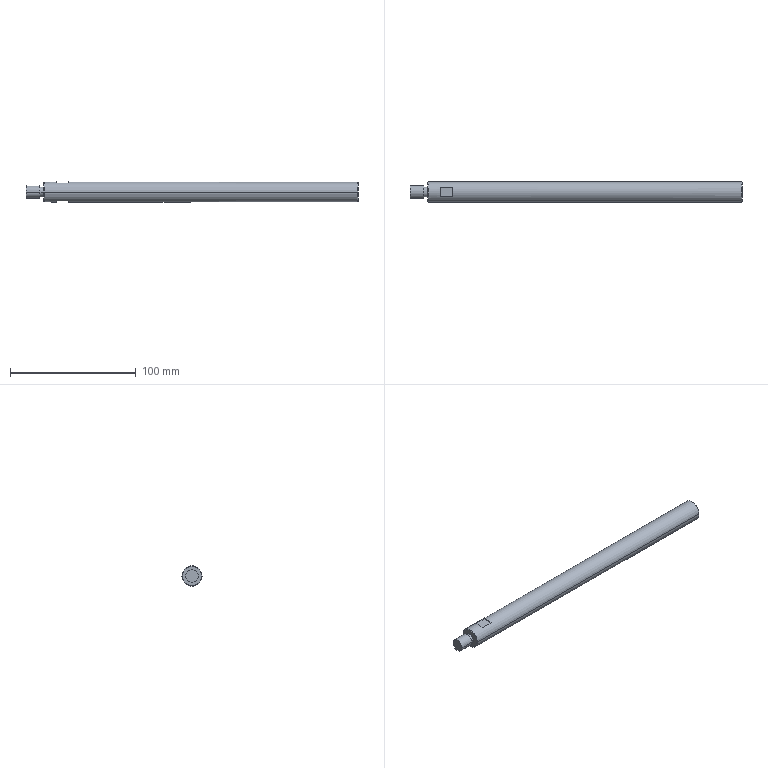Part | STEP file | PSSAGS16-250-F14-M10-SC10 | 1 solid | 20 faces | box 264 x 16 x 16 mm | volume 51157 mm3 | plane 10 | cylinder 6 | cone 4 | commonest cylinder face diameters 7.7 x2 10 x2 16 x2
STEP:
#1=CARTESIAN_POINT('',(0.,0.,0.));
#2=DIRECTION('',(0.,0.,1.));
#3=DIRECTION('',(1.,0.,0.));
#4=AXIS2_PLACEMENT_3D('',#1,#2,#3);
#5=CARTESIAN_POINT('',(264.,7.6,0.));
#6=VERTEX_POINT('',#5);
#7=CARTESIAN_POINT('',(264.,-7.6,0.));
#8=VERTEX_POINT('',#7);
#9=CARTESIAN_POINT('',(264.,0.,0.));
#10=DIRECTION('',(1.,0.,0.));
#11=DIRECTION('',(0.,-1.,0.));
#12=AXIS2_PLACEMENT_3D('',#9,#10,#11);
#13=CIRCLE('',#12,7.6);
#14=CARTESIAN_POINT('',(263.6,0.,0.));
#15=DIRECTION('',(-1.,0.,0.));
#16=DIRECTION('',(0.,-1.,0.));
#17=AXIS2_PLACEMENT_3D('',#14,#15,#16);
#18=CONICAL_SURFACE('',#17,8.,0.7854);
#19=CARTESIAN_POINT('',(6.283,-0.4));
#20=DIRECTION('',(-1.,0.));
#21=VECTOR('',#20,1.);
#22=LINE('',#19,#21);
#23=(GEOMETRIC_REPRESENTATION_CONTEXT(2)PARAMETRIC_REPRESENTATION_CONTEXT()REPRESENTATION_CONTEXT('',''));
#24=DEFINITIONAL_REPRESENTATION('',(#22),#23);
#25=PCURVE('',#18,#24);
#26=CARTESIAN_POINT('',(264.,8.,0.));
#27=DIRECTION('',(-1.,0.,0.));
#28=DIRECTION('',(0.,-1.,0.));
#29=AXIS2_PLACEMENT_3D('',#26,#27,#28);
#30=PLANE('',#29);
#31=CARTESIAN_POINT('',(15.6,0.));
#32=CARTESIAN_POINT('',(15.6,-13.164));
#33=CARTESIAN_POINT('',(4.2,-6.582));
#34=CARTESIAN_POINT('',(-7.2,0.));
#35=CARTESIAN_POINT('',(4.2,6.582));
#36=CARTESIAN_POINT('',(15.6,13.164));
#37=CARTESIAN_POINT('',(15.6,0.));
#38=(BOUNDED_CURVE()B_SPLINE_CURVE(2,(#31,#32,#33,#34,#35,#36,#37),.UNSPECIFIED.,.T.,.F.)B_SPLINE_CURVE_WITH_KNOTS((1,2,2,2,2,1),(-2.094,0.,2.094,4.189,6.283,8.378),.UNSPECIFIED.)CURVE()GEOMETRIC_REPRESENTATION_ITEM()RATIONAL_B_SPLINE_CURVE((1.,0.5,1.,0.5,1.,0.5,1.))REPRESENTATION_ITEM(''));
#39=(GEOMETRIC_REPRESENTATION_CONTEXT(2)PARAMETRIC_REPRESENTATION_CONTEXT()REPRESENTATION_CONTEXT('',''));
#40=DEFINITIONAL_REPRESENTATION('',(#38),#39);
#41=PCURVE('',#30,#40);
#42=SURFACE_CURVE('',#13,(#25,#41),.PCURVE_S1.);
#43=EDGE_CURVE('',#6,#8,#42,.T.);
#44=ORIENTED_EDGE('',*,*,#43,.F.);
#45=CARTESIAN_POINT('',(263.6,8.,0.));
#46=VERTEX_POINT('',#45);
#47=CARTESIAN_POINT('',(263.6,8.,0.));
#48=DIRECTION('',(-0.7071,0.7071,0.));
#49=VECTOR('',#48,1.);
#50=LINE('',#47,#49);
#51=CARTESIAN_POINT('',(3.142,0.));
#52=DIRECTION('',(0.,1.));
#53=VECTOR('',#52,1.);
#54=LINE('',#51,#53);
#55=(GEOMETRIC_REPRESENTATION_CONTEXT(2)PARAMETRIC_REPRESENTATION_CONTEXT()REPRESENTATION_CONTEXT('',''));
#56=DEFINITIONAL_REPRESENTATION('',(#54),#55);
#57=PCURVE('',#18,#56);
#58=CARTESIAN_POINT('',(263.6,0.,0.));
#59=DIRECTION('',(-1.,0.,0.));
#60=DIRECTION('',(0.,-1.,0.));
#61=AXIS2_PLACEMENT_3D('',#58,#59,#60);
#62=CONICAL_SURFACE('',#61,8.,0.7854);
#63=CARTESIAN_POINT('',(3.142,0.));
#64=DIRECTION('',(0.,1.));
#65=VECTOR('',#64,1.);
#66=LINE('',#63,#65);
#67=(GEOMETRIC_REPRESENTATION_CONTEXT(2)PARAMETRIC_REPRESENTATION_CONTEXT()REPRESENTATION_CONTEXT('',''));
#68=DEFINITIONAL_REPRESENTATION('',(#66),#67);
#69=PCURVE('',#62,#68);
#70=SURFACE_CURVE('',#50,(#57,#69),.PCURVE_S1.);
#71=EDGE_CURVE('',#6,#46,#70,.T.);
#72=ORIENTED_EDGE('',*,*,#71,.T.);
#73=CARTESIAN_POINT('',(263.6,-8.,0.));
#74=VERTEX_POINT('',#73);
#75=CARTESIAN_POINT('',(263.6,0.,0.));
#76=DIRECTION('',(-1.,0.,0.));
#77=DIRECTION('',(0.,-1.,0.));
#78=AXIS2_PLACEMENT_3D('',#75,#76,#77);
#79=CIRCLE('',#78,8.);
#80=CARTESIAN_POINT('',(0.,0.));
#81=DIRECTION('',(1.,0.));
#82=VECTOR('',#81,1.);
#83=LINE('',#80,#82);
#84=(GEOMETRIC_REPRESENTATION_CONTEXT(2)PARAMETRIC_REPRESENTATION_CONTEXT()REPRESENTATION_CONTEXT('',''));
#85=DEFINITIONAL_REPRESENTATION('',(#83),#84);
#86=PCURVE('',#18,#85);
#87=CARTESIAN_POINT('',(0.,0.,0.));
#88=DIRECTION('',(-1.,0.,0.));
#89=DIRECTION('',(0.,-1.,0.));
#90=AXIS2_PLACEMENT_3D('',#87,#88,#89);
#91=CYLINDRICAL_SURFACE('',#90,8.);
#92=CARTESIAN_POINT('',(0.,-263.6));
#93=DIRECTION('',(1.,0.));
#94=VECTOR('',#93,1.);
#95=LINE('',#92,#94);
#96=(GEOMETRIC_REPRESENTATION_CONTEXT(2)PARAMETRIC_REPRESENTATION_CONTEXT()REPRESENTATION_CONTEXT('',''));
#97=DEFINITIONAL_REPRESENTATION('',(#95),#96);
#98=PCURVE('',#91,#97);
#99=SURFACE_CURVE('',#79,(#86,#98),.PCURVE_S1.);
#100=EDGE_CURVE('',#74,#46,#99,.T.);
#101=ORIENTED_EDGE('',*,*,#100,.F.);
#102=CARTESIAN_POINT('',(263.6,-8.,0.));
#103=DIRECTION('',(-0.7071,-0.7071,0.));
#104=VECTOR('',#103,1.);
#105=LINE('',#102,#104);
#106=CARTESIAN_POINT('',(0.,0.));
#107=DIRECTION('',(0.,1.));
#108=VECTOR('',#107,1.);
#109=LINE('',#106,#108);
#110=(GEOMETRIC_REPRESENTATION_CONTEXT(2)PARAMETRIC_REPRESENTATION_CONTEXT()REPRESENTATION_CONTEXT('',''));
#111=DEFINITIONAL_REPRESENTATION('',(#109),#110);
#112=PCURVE('',#18,#111);
#113=CARTESIAN_POINT('',(6.283,0.));
#114=DIRECTION('',(0.,1.));
#115=VECTOR('',#114,1.);
#116=LINE('',#113,#115);
#117=(GEOMETRIC_REPRESENTATION_CONTEXT(2)PARAMETRIC_REPRESENTATION_CONTEXT()REPRESENTATION_CONTEXT('',''));
#118=DEFINITIONAL_REPRESENTATION('',(#116),#117);
#119=PCURVE('',#62,#118);
#120=SURFACE_CURVE('',#105,(#112,#119),.PCURVE_S1.);
#121=EDGE_CURVE('',#8,#74,#120,.T.);
#122=ORIENTED_EDGE('',*,*,#121,.F.);
#123=EDGE_LOOP('',(#44,#72,#101,#122));
#124=FACE_BOUND('',#123,.T.);
#125=ADVANCED_FACE('',(#124),#18,.T.);
#126=CARTESIAN_POINT('',(14.,-7.6,0.));
#127=VERTEX_POINT('',#126);
#128=CARTESIAN_POINT('',(14.,7.6,0.));
#129=VERTEX_POINT('',#128);
#130=CARTESIAN_POINT('',(14.,0.,0.));
#131=DIRECTION('',(-1.,0.,0.));
#132=DIRECTION('',(0.,1.,0.));
#133=AXIS2_PLACEMENT_3D('',#130,#131,#132);
#134=CIRCLE('',#133,7.6);
#135=CARTESIAN_POINT('',(14.,0.,0.));
#136=DIRECTION('',(1.,0.,0.));
#137=DIRECTION('',(0.,1.,0.));
#138=AXIS2_PLACEMENT_3D('',#135,#136,#137);
#139=CONICAL_SURFACE('',#138,7.6,0.7854);
#140=CARTESIAN_POINT('',(6.283,0.));
#141=DIRECTION('',(-1.,0.));
#142=VECTOR('',#141,1.);
#143=LINE('',#140,#142);
#144=(GEOMETRIC_REPRESENTATION_CONTEXT(2)PARAMETRIC_REPRESENTATION_CONTEXT()REPRESENTATION_CONTEXT('',''));
#145=DEFINITIONAL_REPRESENTATION('',(#143),#144);
#146=PCURVE('',#139,#145);
#147=CARTESIAN_POINT('',(14.,3.85,0.));
#148=DIRECTION('',(1.,0.,0.));
#149=DIRECTION('',(0.,1.,0.));
#150=AXIS2_PLACEMENT_3D('',#147,#148,#149);
#151=PLANE('',#150);
#152=CARTESIAN_POINT('',(3.75,0.));
#153=CARTESIAN_POINT('',(3.75,-13.164));
#154=CARTESIAN_POINT('',(-7.65,-6.582));
#155=CARTESIAN_POINT('',(-19.05,0.));
#156=CARTESIAN_POINT('',(-7.65,6.582));
#157=CARTESIAN_POINT('',(3.75,13.164));
#158=CARTESIAN_POINT('',(3.75,0.));
#159=(BOUNDED_CURVE()B_SPLINE_CURVE(2,(#152,#153,#154,#155,#156,#157,#158),.UNSPECIFIED.,.T.,.F.)B_SPLINE_CURVE_WITH_KNOTS((1,2,2,2,2,1),(-2.094,0.,2.094,4.189,6.283,8.378),.UNSPECIFIED.)CURVE()GEOMETRIC_REPRESENTATION_ITEM()RATIONAL_B_SPLINE_CURVE((1.,0.5,1.,0.5,1.,0.5,1.))REPRESENTATION_ITEM(''));
#160=(GEOMETRIC_REPRESENTATION_CONTEXT(2)PARAMETRIC_REPRESENTATION_CONTEXT()REPRESENTATION_CONTEXT('',''));
#161=DEFINITIONAL_REPRESENTATION('',(#159),#160);
#162=PCURVE('',#151,#161);
#163=SURFACE_CURVE('',#134,(#146,#162),.PCURVE_S1.);
#164=EDGE_CURVE('',#127,#129,#163,.T.);
#165=ORIENTED_EDGE('',*,*,#164,.F.);
#166=CARTESIAN_POINT('',(14.4,-8.,0.));
#167=VERTEX_POINT('',#166);
#168=CARTESIAN_POINT('',(14.,-7.6,0.));
#169=DIRECTION('',(0.7071,-0.7071,0.));
#170=VECTOR('',#169,1.);
#171=LINE('',#168,#170);
#172=CARTESIAN_POINT('',(3.142,0.));
#173=DIRECTION('',(0.,1.));
#174=VECTOR('',#173,1.);
#175=LINE('',#172,#174);
#176=(GEOMETRIC_REPRESENTATION_CONTEXT(2)PARAMETRIC_REPRESENTATION_CONTEXT()REPRESENTATION_CONTEXT('',''));
#177=DEFINITIONAL_REPRESENTATION('',(#175),#176);
#178=PCURVE('',#139,#177);
#179=CARTESIAN_POINT('',(14.,0.,0.));
#180=DIRECTION('',(1.,0.,0.));
#181=DIRECTION('',(0.,1.,0.));
#182=AXIS2_PLACEMENT_3D('',#179,#180,#181);
#183=CONICAL_SURFACE('',#182,7.6,0.7854);
#184=CARTESIAN_POINT('',(3.142,0.));
#185=DIRECTION('',(0.,1.));
#186=VECTOR('',#185,1.);
#187=LINE('',#184,#186);
#188=(GEOMETRIC_REPRESENTATION_CONTEXT(2)PARAMETRIC_REPRESENTATION_CONTEXT()REPRESENTATION_CONTEXT('',''));
#189=DEFINITIONAL_REPRESENTATION('',(#187),#188);
#190=PCURVE('',#183,#189);
#191=SURFACE_CURVE('',#171,(#178,#190),.PCURVE_S1.);
#192=EDGE_CURVE('',#127,#167,#191,.T.);
#193=ORIENTED_EDGE('',*,*,#192,.T.);
#194=CARTESIAN_POINT('',(14.4,8.,0.));
#195=VERTEX_POINT('',#194);
#196=CARTESIAN_POINT('',(14.4,0.,0.));
#197=DIRECTION('',(1.,0.,0.));
#198=DIRECTION('',(0.,1.,0.));
#199=AXIS2_PLACEMENT_3D('',#196,#197,#198);
#200=CIRCLE('',#199,8.);
#201=CARTESIAN_POINT('',(0.,0.4));
#202=DIRECTION('',(1.,0.));
#203=VECTOR('',#202,1.);
#204=LINE('',#201,#203);
#205=(GEOMETRIC_REPRESENTATION_CONTEXT(2)PARAMETRIC_REPRESENTATION_CONTEXT()REPRESENTATION_CONTEXT('',''));
#206=DEFINITIONAL_REPRESENTATION('',(#204),#205);
#207=PCURVE('',#139,#206);
#208=CARTESIAN_POINT('',(3.142,-14.4));
#209=DIRECTION('',(-1.,0.));
#210=VECTOR('',#209,1.);
#211=LINE('',#208,#210);
#212=(GEOMETRIC_REPRESENTATION_CONTEXT(2)PARAMETRIC_REPRESENTATION_CONTEXT()REPRESENTATION_CONTEXT('',''));
#213=DEFINITIONAL_REPRESENTATION('',(#211),#212);
#214=PCURVE('',#91,#213);
#215=SURFACE_CURVE('',#200,(#207,#214),.PCURVE_S1.);
#216=EDGE_CURVE('',#195,#167,#215,.T.);
#217=ORIENTED_EDGE('',*,*,#216,.F.);
#218=CARTESIAN_POINT('',(14.,7.6,0.));
#219=DIRECTION('',(0.7071,0.7071,0.));
#220=VECTOR('',#219,1.);
#221=LINE('',#218,#220);
#222=CARTESIAN_POINT('',(0.,0.));
#223=DIRECTION('',(0.,1.));
#224=VECTOR('',#223,1.);
#225=LINE('',#222,#224);
#226=(GEOMETRIC_REPRESENTATION_CONTEXT(2)PARAMETRIC_REPRESENTATION_CONTEXT()REPRESENTATION_CONTEXT('',''));
#227=DEFINITIONAL_REPRESENTATION('',(#225),#226);
#228=PCURVE('',#139,#227);
#229=CARTESIAN_POINT('',(6.283,0.));
#230=DIRECTION('',(0.,1.));
#231=VECTOR('',#230,1.);
#232=LINE('',#229,#231);
#233=(GEOMETRIC_REPRESENTATION_CONTEXT(2)PARAMETRIC_REPRESENTATION_CONTEXT()REPRESENTATION_CONTEXT('',''));
#234=DEFINITIONAL_REPRESENTATION('',(#232),#233);
#235=PCURVE('',#183,#234);
#236=SURFACE_CURVE('',#221,(#228,#235),.PCURVE_S1.);
#237=EDGE_CURVE('',#129,#195,#236,.T.);
#238=ORIENTED_EDGE('',*,*,#237,.F.);
#239=EDGE_LOOP('',(#165,#193,#217,#238));
#240=FACE_BOUND('',#239,.T.);
#241=ADVANCED_FACE('',(#240),#139,.T.);
#242=CARTESIAN_POINT('',(24.,3.873,7.));
#243=VERTEX_POINT('',#242);
#244=CARTESIAN_POINT('',(34.,3.873,7.));
#245=VERTEX_POINT('',#244);
#246=CARTESIAN_POINT('',(0.,3.873,7.));
#247=DIRECTION('',(1.,0.,0.));
#248=VECTOR('',#247,1.);
#249=LINE('',#246,#248);
#250=CARTESIAN_POINT('',(2.076,0.));
#251=DIRECTION('',(0.,-1.));
#252=VECTOR('',#251,1.);
#253=LINE('',#250,#252);
#254=(GEOMETRIC_REPRESENTATION_CONTEXT(2)PARAMETRIC_REPRESENTATION_CONTEXT()REPRESENTATION_CONTEXT('',''));
#255=DEFINITIONAL_REPRESENTATION('',(#253),#254);
#256=PCURVE('',#91,#255);
#257=CARTESIAN_POINT('',(24.,-8.,7.));
#258=DIRECTION('',(0.,0.,-1.));
#259=DIRECTION('',(-1.,0.,0.));
#260=AXIS2_PLACEMENT_3D('',#257,#258,#259);
#261=PLANE('',#260);
#262=CARTESIAN_POINT('',(24.,11.873));
#263=DIRECTION('',(-1.,0.));
#264=VECTOR('',#263,1.);
#265=LINE('',#262,#264);
#266=(GEOMETRIC_REPRESENTATION_CONTEXT(2)PARAMETRIC_REPRESENTATION_CONTEXT()REPRESENTATION_CONTEXT('',''));
#267=DEFINITIONAL_REPRESENTATION('',(#265),#266);
#268=PCURVE('',#261,#267);
#269=SURFACE_CURVE('',#249,(#256,#268),.PCURVE_S1.);
#270=EDGE_CURVE('',#243,#245,#269,.T.);
#271=ORIENTED_EDGE('',*,*,#270,.T.);
#272=CARTESIAN_POINT('',(34.,-3.873,7.));
#273=VERTEX_POINT('',#272);
#274=CARTESIAN_POINT('',(34.,0.,0.));
#275=DIRECTION('',(1.,0.,0.));
#276=DIRECTION('',(0.,0.,-1.));
#277=AXIS2_PLACEMENT_3D('',#274,#275,#276);
#278=CIRCLE('',#277,8.);
#279=CARTESIAN_POINT('',(4.712,-34.));
#280=DIRECTION('',(-1.,0.));
#281=VECTOR('',#280,1.);
#282=LINE('',#279,#281);
#283=(GEOMETRIC_REPRESENTATION_CONTEXT(2)PARAMETRIC_REPRESENTATION_CONTEXT()REPRESENTATION_CONTEXT('',''));
#284=DEFINITIONAL_REPRESENTATION('',(#282),#283);
#285=PCURVE('',#91,#284);
#286=CARTESIAN_POINT('',(34.,-8.,7.));
#287=DIRECTION('',(1.,0.,0.));
#288=DIRECTION('',(0.,0.,-1.));
#289=AXIS2_PLACEMENT_3D('',#286,#287,#288);
#290=PLANE('',#289);
#291=CARTESIAN_POINT('',(7.,8.));
#292=DIRECTION('',(1.,0.));
#293=AXIS2_PLACEMENT_2D('',#291,#292);
#294=CIRCLE('',#293,8.);
#295=(GEOMETRIC_REPRESENTATION_CONTEXT(2)PARAMETRIC_REPRESENTATION_CONTEXT()REPRESENTATION_CONTEXT('',''));
#296=DEFINITIONAL_REPRESENTATION('',(#294),#295);
#297=PCURVE('',#290,#296);
#298=SURFACE_CURVE('',#278,(#285,#297),.PCURVE_S1.);
#299=EDGE_CURVE('',#245,#273,#298,.T.);
#300=ORIENTED_EDGE('',*,*,#299,.T.);
#301=CARTESIAN_POINT('',(24.,-3.873,7.));
#302=VERTEX_POINT('',#301);
#303=CARTESIAN_POINT('',(0.,-3.873,7.));
#304=DIRECTION('',(-1.,0.,0.));
#305=VECTOR('',#304,1.);
#306=LINE('',#303,#305);
#307=CARTESIAN_POINT('',(1.065,0.));
#308=DIRECTION('',(0.,1.));
#309=VECTOR('',#308,1.);
#310=LINE('',#307,#309);
#311=(GEOMETRIC_REPRESENTATION_CONTEXT(2)PARAMETRIC_REPRESENTATION_CONTEXT()REPRESENTATION_CONTEXT('',''));
#312=DEFINITIONAL_REPRESENTATION('',(#310),#311);
#313=PCURVE('',#91,#312);
#314=CARTESIAN_POINT('',(24.,4.127));
#315=DIRECTION('',(1.,0.));
#316=VECTOR('',#315,1.);
#317=LINE('',#314,#316);
#318=(GEOMETRIC_REPRESENTATION_CONTEXT(2)PARAMETRIC_REPRESENTATION_CONTEXT()REPRESENTATION_CONTEXT('',''));
#319=DEFINITIONAL_REPRESENTATION('',(#317),#318);
#320=PCURVE('',#261,#319);
#321=SURFACE_CURVE('',#306,(#313,#320),.PCURVE_S1.);
#322=EDGE_CURVE('',#273,#302,#321,.T.);
#323=ORIENTED_EDGE('',*,*,#322,.T.);
#324=CARTESIAN_POINT('',(24.,0.,0.));
#325=DIRECTION('',(-1.,0.,0.));
#326=DIRECTION('',(0.,0.,1.));
#327=AXIS2_PLACEMENT_3D('',#324,#325,#326);
#328=CIRCLE('',#327,8.);
#329=CARTESIAN_POINT('',(-4.712,-24.));
#330=DIRECTION('',(1.,0.));
#331=VECTOR('',#330,1.);
#332=LINE('',#329,#331);
#333=(GEOMETRIC_REPRESENTATION_CONTEXT(2)PARAMETRIC_REPRESENTATION_CONTEXT()REPRESENTATION_CONTEXT('',''));
#334=DEFINITIONAL_REPRESENTATION('',(#332),#333);
#335=PCURVE('',#91,#334);
#336=CARTESIAN_POINT('',(24.,-8.,7.));
#337=DIRECTION('',(-1.,0.,0.));
#338=DIRECTION('',(0.,0.,1.));
#339=AXIS2_PLACEMENT_3D('',#336,#337,#338);
#340=PLANE('',#339);
#341=CARTESIAN_POINT('',(-7.,8.));
#342=DIRECTION('',(1.,0.));
#343=AXIS2_PLACEMENT_2D('',#341,#342);
#344=CIRCLE('',#343,8.);
#345=(GEOMETRIC_REPRESENTATION_CONTEXT(2)PARAMETRIC_REPRESENTATION_CONTEXT()REPRESENTATION_CONTEXT('',''));
#346=DEFINITIONAL_REPRESENTATION('',(#344),#345);
#347=PCURVE('',#340,#346);
#348=SURFACE_CURVE('',#328,(#335,#347),.PCURVE_S1.);
#349=EDGE_CURVE('',#302,#243,#348,.T.);
#350=ORIENTED_EDGE('',*,*,#349,.T.);
#351=EDGE_LOOP('',(#271,#300,#323,#350));
#352=FACE_BOUND('',#351,.T.);
#353=ORIENTED_EDGE('',*,*,#100,.T.);
#354=CARTESIAN_POINT('',(0.,8.,0.));
#355=DIRECTION('',(-1.,0.,0.));
#356=VECTOR('',#355,1.);
#357=LINE('',#354,#356);
#358=CARTESIAN_POINT('',(3.142,0.));
#359=DIRECTION('',(0.,1.));
#360=VECTOR('',#359,1.);
#361=LINE('',#358,#360);
#362=(GEOMETRIC_REPRESENTATION_CONTEXT(2)PARAMETRIC_REPRESENTATION_CONTEXT()REPRESENTATION_CONTEXT('',''));
#363=DEFINITIONAL_REPRESENTATION('',(#361),#362);
#364=PCURVE('',#91,#363);
#365=CARTESIAN_POINT('',(0.,0.,0.));
#366=DIRECTION('',(-1.,0.,0.));
#367=DIRECTION('',(0.,-1.,0.));
#368=AXIS2_PLACEMENT_3D('',#365,#366,#367);
#369=CYLINDRICAL_SURFACE('',#368,8.);
#370=CARTESIAN_POINT('',(3.142,0.));
#371=DIRECTION('',(0.,1.));
#372=VECTOR('',#371,1.);
#373=LINE('',#370,#372);
#374=(GEOMETRIC_REPRESENTATION_CONTEXT(2)PARAMETRIC_REPRESENTATION_CONTEXT()REPRESENTATION_CONTEXT('',''));
#375=DEFINITIONAL_REPRESENTATION('',(#373),#374);
#376=PCURVE('',#369,#375);
#377=SURFACE_CURVE('',#357,(#364,#376),.PCURVE_S1.);
#378=EDGE_CURVE('',#46,#195,#377,.T.);
#379=ORIENTED_EDGE('',*,*,#378,.T.);
#380=ORIENTED_EDGE('',*,*,#216,.T.);
#381=CARTESIAN_POINT('',(0.,-8.,0.));
#382=DIRECTION('',(-1.,0.,0.));
#383=VECTOR('',#382,1.);
#384=LINE('',#381,#383);
#385=CARTESIAN_POINT('',(0.,0.));
#386=DIRECTION('',(0.,1.));
#387=VECTOR('',#386,1.);
#388=LINE('',#385,#387);
#389=(GEOMETRIC_REPRESENTATION_CONTEXT(2)PARAMETRIC_REPRESENTATION_CONTEXT()REPRESENTATION_CONTEXT('',''));
#390=DEFINITIONAL_REPRESENTATION('',(#388),#389);
#391=PCURVE('',#91,#390);
#392=CARTESIAN_POINT('',(6.283,0.));
#393=DIRECTION('',(0.,1.));
#394=VECTOR('',#393,1.);
#395=LINE('',#392,#394);
#396=(GEOMETRIC_REPRESENTATION_CONTEXT(2)PARAMETRIC_REPRESENTATION_CONTEXT()REPRESENTATION_CONTEXT('',''));
#397=DEFINITIONAL_REPRESENTATION('',(#395),#396);
#398=PCURVE('',#369,#397);
#399=SURFACE_CURVE('',#384,(#391,#398),.PCURVE_S1.);
#400=EDGE_CURVE('',#74,#167,#399,.T.);
#401=ORIENTED_EDGE('',*,*,#400,.F.);
#402=EDGE_LOOP('',(#353,#379,#380,#401));
#403=FACE_BOUND('',#402,.T.);
#404=ADVANCED_FACE('',(#352,#403),#91,.T.);
#405=CARTESIAN_POINT('',(14.,-3.85,0.));
#406=VERTEX_POINT('',#405);
#407=CARTESIAN_POINT('',(14.,3.85,0.));
#408=VERTEX_POINT('',#407);
#409=CARTESIAN_POINT('',(14.,0.,0.));
#410=DIRECTION('',(-1.,0.,0.));
#411=DIRECTION('',(0.,-1.,0.));
#412=AXIS2_PLACEMENT_3D('',#409,#410,#411);
#413=CIRCLE('',#412,3.85);
#414=CARTESIAN_POINT('',(0.,0.,0.));
#415=DIRECTION('',(-1.,0.,0.));
#416=DIRECTION('',(0.,-1.,0.));
#417=AXIS2_PLACEMENT_3D('',#414,#415,#416);
#418=CYLINDRICAL_SURFACE('',#417,3.85);
#419=CARTESIAN_POINT('',(0.,-14.));
#420=DIRECTION('',(1.,0.));
#421=VECTOR('',#420,1.);
#422=LINE('',#419,#421);
#423=(GEOMETRIC_REPRESENTATION_CONTEXT(2)PARAMETRIC_REPRESENTATION_CONTEXT()REPRESENTATION_CONTEXT('',''));
#424=DEFINITIONAL_REPRESENTATION('',(#422),#423);
#425=PCURVE('',#418,#424);
#426=CARTESIAN_POINT('',(-7.7,0.));
#427=CARTESIAN_POINT('',(-7.7,6.668));
#428=CARTESIAN_POINT('',(-1.925,3.334));
#429=CARTESIAN_POINT('',(3.85,0.));
#430=CARTESIAN_POINT('',(-1.925,-3.334));
#431=CARTESIAN_POINT('',(-7.7,-6.668));
#432=CARTESIAN_POINT('',(-7.7,0.));
#433=(BOUNDED_CURVE()B_SPLINE_CURVE(2,(#426,#427,#428,#429,#430,#431,#432),.UNSPECIFIED.,.T.,.F.)B_SPLINE_CURVE_WITH_KNOTS((1,2,2,2,2,1),(-2.094,0.,2.094,4.189,6.283,8.378),.UNSPECIFIED.)CURVE()GEOMETRIC_REPRESENTATION_ITEM()RATIONAL_B_SPLINE_CURVE((1.,0.5,1.,0.5,1.,0.5,1.))REPRESENTATION_ITEM(''));
#434=(GEOMETRIC_REPRESENTATION_CONTEXT(2)PARAMETRIC_REPRESENTATION_CONTEXT()REPRESENTATION_CONTEXT('',''));
#435=DEFINITIONAL_REPRESENTATION('',(#433),#434);
#436=PCURVE('',#151,#435);
#437=SURFACE_CURVE('',#413,(#425,#436),.PCURVE_S1.);
#438=EDGE_CURVE('',#406,#408,#437,.T.);
#439=ORIENTED_EDGE('',*,*,#438,.T.);
#440=CARTESIAN_POINT('',(11.,3.85,0.));
#441=VERTEX_POINT('',#440);
#442=CARTESIAN_POINT('',(0.,3.85,0.));
#443=DIRECTION('',(-1.,0.,0.));
#444=VECTOR('',#443,1.);
#445=LINE('',#442,#444);
#446=CARTESIAN_POINT('',(3.142,0.));
#447=DIRECTION('',(0.,1.));
#448=VECTOR('',#447,1.);
#449=LINE('',#446,#448);
#450=(GEOMETRIC_REPRESENTATION_CONTEXT(2)PARAMETRIC_REPRESENTATION_CONTEXT()REPRESENTATION_CONTEXT('',''));
#451=DEFINITIONAL_REPRESENTATION('',(#449),#450);
#452=PCURVE('',#418,#451);
#453=CARTESIAN_POINT('',(0.,0.,0.));
#454=DIRECTION('',(-1.,0.,0.));
#455=DIRECTION('',(0.,-1.,0.));
#456=AXIS2_PLACEMENT_3D('',#453,#454,#455);
#457=CYLINDRICAL_SURFACE('',#456,3.85);
#458=CARTESIAN_POINT('',(3.142,0.));
#459=DIRECTION('',(0.,1.));
#460=VECTOR('',#459,1.);
#461=LINE('',#458,#460);
#462=(GEOMETRIC_REPRESENTATION_CONTEXT(2)PARAMETRIC_REPRESENTATION_CONTEXT()REPRESENTATION_CONTEXT('',''));
#463=DEFINITIONAL_REPRESENTATION('',(#461),#462);
#464=PCURVE('',#457,#463);
#465=SURFACE_CURVE('',#445,(#452,#464),.PCURVE_S1.);
#466=EDGE_CURVE('',#408,#441,#465,.T.);
#467=ORIENTED_EDGE('',*,*,#466,.T.);
#468=CARTESIAN_POINT('',(11.,-3.85,0.));
#469=VERTEX_POINT('',#468);
#470=CARTESIAN_POINT('',(11.,0.,0.));
#471=DIRECTION('',(-1.,0.,0.));
#472=DIRECTION('',(0.,-1.,0.));
#473=AXIS2_PLACEMENT_3D('',#470,#471,#472);
#474=CIRCLE('',#473,3.85);
#475=CARTESIAN_POINT('',(0.,-11.));
#476=DIRECTION('',(1.,0.));
#477=VECTOR('',#476,1.);
#478=LINE('',#475,#477);
#479=(GEOMETRIC_REPRESENTATION_CONTEXT(2)PARAMETRIC_REPRESENTATION_CONTEXT()REPRESENTATION_CONTEXT('',''));
#480=DEFINITIONAL_REPRESENTATION('',(#478),#479);
#481=PCURVE('',#418,#480);
#482=CARTESIAN_POINT('',(11.,5.,0.));
#483=DIRECTION('',(-1.,0.,0.));
#484=DIRECTION('',(0.,-1.,0.));
#485=AXIS2_PLACEMENT_3D('',#482,#483,#484);
#486=PLANE('',#485);
#487=CARTESIAN_POINT('',(5.,0.));
#488=DIRECTION('',(1.,0.));
#489=AXIS2_PLACEMENT_2D('',#487,#488);
#490=CIRCLE('',#489,3.85);
#491=(GEOMETRIC_REPRESENTATION_CONTEXT(2)PARAMETRIC_REPRESENTATION_CONTEXT()REPRESENTATION_CONTEXT('',''));
#492=DEFINITIONAL_REPRESENTATION('',(#490),#491);
#493=PCURVE('',#486,#492);
#494=SURFACE_CURVE('',#474,(#481,#493),.PCURVE_S1.);
#495=EDGE_CURVE('',#469,#441,#494,.T.);
#496=ORIENTED_EDGE('',*,*,#495,.F.);
#497=CARTESIAN_POINT('',(0.,-3.85,0.));
#498=DIRECTION('',(-1.,0.,0.));
#499=VECTOR('',#498,1.);
#500=LINE('',#497,#499);
#501=CARTESIAN_POINT('',(0.,0.));
#502=DIRECTION('',(0.,1.));
#503=VECTOR('',#502,1.);
#504=LINE('',#501,#503);
#505=(GEOMETRIC_REPRESENTATION_CONTEXT(2)PARAMETRIC_REPRESENTATION_CONTEXT()REPRESENTATION_CONTEXT('',''));
#506=DEFINITIONAL_REPRESENTATION('',(#504),#505);
#507=PCURVE('',#418,#506);
#508=CARTESIAN_POINT('',(6.283,0.));
#509=DIRECTION('',(0.,1.));
#510=VECTOR('',#509,1.);
#511=LINE('',#508,#510);
#512=(GEOMETRIC_REPRESENTATION_CONTEXT(2)PARAMETRIC_REPRESENTATION_CONTEXT()REPRESENTATION_CONTEXT('',''));
#513=DEFINITIONAL_REPRESENTATION('',(#511),#512);
#514=PCURVE('',#457,#513);
#515=SURFACE_CURVE('',#500,(#507,#514),.PCURVE_S1.);
#516=EDGE_CURVE('',#406,#469,#515,.T.);
#517=ORIENTED_EDGE('',*,*,#516,.F.);
#518=EDGE_LOOP('',(#439,#467,#496,#517));
#519=FACE_BOUND('',#518,.T.);
#520=ADVANCED_FACE('',(#519),#418,.T.);
#521=CARTESIAN_POINT('',(11.,-5.,0.));
#522=VERTEX_POINT('',#521);
#523=CARTESIAN_POINT('',(11.,5.,0.));
#524=VERTEX_POINT('',#523);
#525=CARTESIAN_POINT('',(11.,0.,0.));
#526=DIRECTION('',(-1.,0.,0.));
#527=DIRECTION('',(0.,-1.,0.));
#528=AXIS2_PLACEMENT_3D('',#525,#526,#527);
#529=CIRCLE('',#528,5.);
#530=CARTESIAN_POINT('',(0.,0.,0.));
#531=DIRECTION('',(-1.,0.,0.));
#532=DIRECTION('',(0.,-1.,0.));
#533=AXIS2_PLACEMENT_3D('',#530,#531,#532);
#534=CYLINDRICAL_SURFACE('',#533,5.);
#535=CARTESIAN_POINT('',(0.,-11.));
#536=DIRECTION('',(1.,0.));
#537=VECTOR('',#536,1.);
#538=LINE('',#535,#537);
#539=(GEOMETRIC_REPRESENTATION_CONTEXT(2)PARAMETRIC_REPRESENTATION_CONTEXT()REPRESENTATION_CONTEXT('',''));
#540=DEFINITIONAL_REPRESENTATION('',(#538),#539);
#541=PCURVE('',#534,#540);
#542=CARTESIAN_POINT('',(5.,0.));
#543=DIRECTION('',(1.,0.));
#544=AXIS2_PLACEMENT_2D('',#542,#543);
#545=CIRCLE('',#544,5.);
#546=(GEOMETRIC_REPRESENTATION_CONTEXT(2)PARAMETRIC_REPRESENTATION_CONTEXT()REPRESENTATION_CONTEXT('',''));
#547=DEFINITIONAL_REPRESENTATION('',(#545),#546);
#548=PCURVE('',#486,#547);
#549=SURFACE_CURVE('',#529,(#541,#548),.PCURVE_S1.);
#550=EDGE_CURVE('',#522,#524,#549,.T.);
#551=ORIENTED_EDGE('',*,*,#550,.T.);
#552=CARTESIAN_POINT('',(0.,5.,0.));
#553=VERTEX_POINT('',#552);
#554=CARTESIAN_POINT('',(0.,5.,0.));
#555=DIRECTION('',(-1.,0.,0.));
#556=VECTOR('',#555,1.);
#557=LINE('',#554,#556);
#558=CARTESIAN_POINT('',(3.142,0.));
#559=DIRECTION('',(0.,1.));
#560=VECTOR('',#559,1.);
#561=LINE('',#558,#560);
#562=(GEOMETRIC_REPRESENTATION_CONTEXT(2)PARAMETRIC_REPRESENTATION_CONTEXT()REPRESENTATION_CONTEXT('',''));
#563=DEFINITIONAL_REPRESENTATION('',(#561),#562);
#564=PCURVE('',#534,#563);
#565=CARTESIAN_POINT('',(0.,0.,0.));
#566=DIRECTION('',(-1.,0.,0.));
#567=DIRECTION('',(0.,-1.,0.));
#568=AXIS2_PLACEMENT_3D('',#565,#566,#567);
#569=CYLINDRICAL_SURFACE('',#568,5.);
#570=CARTESIAN_POINT('',(3.142,0.));
#571=DIRECTION('',(0.,1.));
#572=VECTOR('',#571,1.);
#573=LINE('',#570,#572);
#574=(GEOMETRIC_REPRESENTATION_CONTEXT(2)PARAMETRIC_REPRESENTATION_CONTEXT()REPRESENTATION_CONTEXT('',''));
#575=DEFINITIONAL_REPRESENTATION('',(#573),#574);
#576=PCURVE('',#569,#575);
#577=SURFACE_CURVE('',#557,(#564,#576),.PCURVE_S1.);
#578=EDGE_CURVE('',#524,#553,#577,.T.);
#579=ORIENTED_EDGE('',*,*,#578,.T.);
#580=CARTESIAN_POINT('',(0.,-5.,0.));
#581=VERTEX_POINT('',#580);
#582=CARTESIAN_POINT('',(0.,0.,0.));
#583=DIRECTION('',(-1.,0.,0.));
#584=DIRECTION('',(0.,-1.,0.));
#585=AXIS2_PLACEMENT_3D('',#582,#583,#584);
#586=CIRCLE('',#585,5.);
#587=CARTESIAN_POINT('',(0.,0.));
#588=DIRECTION('',(1.,0.));
#589=VECTOR('',#588,1.);
#590=LINE('',#587,#589);
#591=(GEOMETRIC_REPRESENTATION_CONTEXT(2)PARAMETRIC_REPRESENTATION_CONTEXT()REPRESENTATION_CONTEXT('',''));
#592=DEFINITIONAL_REPRESENTATION('',(#590),#591);
#593=PCURVE('',#534,#592);
#594=CARTESIAN_POINT('',(0.,0.,0.));
#595=DIRECTION('',(1.,0.,0.));
#596=DIRECTION('',(0.,1.,0.));
#597=AXIS2_PLACEMENT_3D('',#594,#595,#596);
#598=PLANE('',#597);
#599=CARTESIAN_POINT('',(-5.,0.));
#600=CARTESIAN_POINT('',(-5.,8.66));
#601=CARTESIAN_POINT('',(2.5,4.33));
#602=CARTESIAN_POINT('',(10.,0.));
#603=CARTESIAN_POINT('',(2.5,-4.33));
#604=CARTESIAN_POINT('',(-5.,-8.66));
#605=CARTESIAN_POINT('',(-5.,0.));
#606=(BOUNDED_CURVE()B_SPLINE_CURVE(2,(#599,#600,#601,#602,#603,#604,#605),.UNSPECIFIED.,.T.,.F.)B_SPLINE_CURVE_WITH_KNOTS((1,2,2,2,2,1),(-2.094,0.,2.094,4.189,6.283,8.378),.UNSPECIFIED.)CURVE()GEOMETRIC_REPRESENTATION_ITEM()RATIONAL_B_SPLINE_CURVE((1.,0.5,1.,0.5,1.,0.5,1.))REPRESENTATION_ITEM(''));
#607=(GEOMETRIC_REPRESENTATION_CONTEXT(2)PARAMETRIC_REPRESENTATION_CONTEXT()REPRESENTATION_CONTEXT('',''));
#608=DEFINITIONAL_REPRESENTATION('',(#606),#607);
#609=PCURVE('',#598,#608);
#610=SURFACE_CURVE('',#586,(#593,#609),.PCURVE_S1.);
#611=EDGE_CURVE('',#581,#553,#610,.T.);
#612=ORIENTED_EDGE('',*,*,#611,.F.);
#613=CARTESIAN_POINT('',(0.,-5.,0.));
#614=DIRECTION('',(-1.,0.,0.));
#615=VECTOR('',#614,1.);
#616=LINE('',#613,#615);
#617=CARTESIAN_POINT('',(0.,0.));
#618=DIRECTION('',(0.,1.));
#619=VECTOR('',#618,1.);
#620=LINE('',#617,#619);
#621=(GEOMETRIC_REPRESENTATION_CONTEXT(2)PARAMETRIC_REPRESENTATION_CONTEXT()REPRESENTATION_CONTEXT('',''));
#622=DEFINITIONAL_REPRESENTATION('',(#620),#621);
#623=PCURVE('',#534,#622);
#624=CARTESIAN_POINT('',(6.283,0.));
#625=DIRECTION('',(0.,1.));
#626=VECTOR('',#625,1.);
#627=LINE('',#624,#626);
#628=(GEOMETRIC_REPRESENTATION_CONTEXT(2)PARAMETRIC_REPRESENTATION_CONTEXT()REPRESENTATION_CONTEXT('',''));
#629=DEFINITIONAL_REPRESENTATION('',(#627),#628);
#630=PCURVE('',#569,#629);
#631=SURFACE_CURVE('',#616,(#623,#630),.PCURVE_S1.);
#632=EDGE_CURVE('',#522,#581,#631,.T.);
#633=ORIENTED_EDGE('',*,*,#632,.F.);
#634=EDGE_LOOP('',(#551,#579,#612,#633));
#635=FACE_BOUND('',#634,.T.);
#636=ADVANCED_FACE('',(#635),#534,.T.);
#637=ORIENTED_EDGE('',*,*,#611,.T.);
#638=CARTESIAN_POINT('',(0.,0.,0.));
#639=DIRECTION('',(-1.,0.,0.));
#640=DIRECTION('',(0.,-1.,0.));
#641=AXIS2_PLACEMENT_3D('',#638,#639,#640);
#642=CIRCLE('',#641,5.);
#643=CARTESIAN_POINT('',(-5.,0.));
#644=CARTESIAN_POINT('',(-5.,8.66));
#645=CARTESIAN_POINT('',(2.5,4.33));
#646=CARTESIAN_POINT('',(10.,0.));
#647=CARTESIAN_POINT('',(2.5,-4.33));
#648=CARTESIAN_POINT('',(-5.,-8.66));
#649=CARTESIAN_POINT('',(-5.,0.));
#650=(BOUNDED_CURVE()B_SPLINE_CURVE(2,(#643,#644,#645,#646,#647,#648,#649),.UNSPECIFIED.,.T.,.F.)B_SPLINE_CURVE_WITH_KNOTS((1,2,2,2,2,1),(-2.094,0.,2.094,4.189,6.283,8.378),.UNSPECIFIED.)CURVE()GEOMETRIC_REPRESENTATION_ITEM()RATIONAL_B_SPLINE_CURVE((1.,0.5,1.,0.5,1.,0.5,1.))REPRESENTATION_ITEM(''));
#651=(GEOMETRIC_REPRESENTATION_CONTEXT(2)PARAMETRIC_REPRESENTATION_CONTEXT()REPRESENTATION_CONTEXT('',''));
#652=DEFINITIONAL_REPRESENTATION('',(#650),#651);
#653=PCURVE('',#598,#652);
#654=CARTESIAN_POINT('',(0.,0.));
#655=DIRECTION('',(1.,0.));
#656=VECTOR('',#655,1.);
#657=LINE('',#654,#656);
#658=(GEOMETRIC_REPRESENTATION_CONTEXT(2)PARAMETRIC_REPRESENTATION_CONTEXT()REPRESENTATION_CONTEXT('',''));
#659=DEFINITIONAL_REPRESENTATION('',(#657),#658);
#660=PCURVE('',#569,#659);
#661=SURFACE_CURVE('',#642,(#653,#660),.PCURVE_S1.);
#662=EDGE_CURVE('',#553,#581,#661,.T.);
#663=ORIENTED_EDGE('',*,*,#662,.T.);
#664=EDGE_LOOP('',(#637,#663));
#665=FACE_BOUND('',#664,.T.);
#666=ADVANCED_FACE('',(#665),#598,.F.);
#667=ORIENTED_EDGE('',*,*,#578,.F.);
#668=CARTESIAN_POINT('',(11.,0.,0.));
#669=DIRECTION('',(-1.,0.,0.));
#670=DIRECTION('',(0.,-1.,0.));
#671=AXIS2_PLACEMENT_3D('',#668,#669,#670);
#672=CIRCLE('',#671,5.);
#673=CARTESIAN_POINT('',(0.,-11.));
#674=DIRECTION('',(1.,0.));
#675=VECTOR('',#674,1.);
#676=LINE('',#673,#675);
#677=(GEOMETRIC_REPRESENTATION_CONTEXT(2)PARAMETRIC_REPRESENTATION_CONTEXT()REPRESENTATION_CONTEXT('',''));
#678=DEFINITIONAL_REPRESENTATION('',(#676),#677);
#679=PCURVE('',#569,#678);
#680=CARTESIAN_POINT('',(5.,0.));
#681=DIRECTION('',(1.,0.));
#682=AXIS2_PLACEMENT_2D('',#680,#681);
#683=CIRCLE('',#682,5.);
#684=(GEOMETRIC_REPRESENTATION_CONTEXT(2)PARAMETRIC_REPRESENTATION_CONTEXT()REPRESENTATION_CONTEXT('',''));
#685=DEFINITIONAL_REPRESENTATION('',(#683),#684);
#686=PCURVE('',#486,#685);
#687=SURFACE_CURVE('',#672,(#679,#686),.PCURVE_S1.);
#688=EDGE_CURVE('',#524,#522,#687,.T.);
#689=ORIENTED_EDGE('',*,*,#688,.T.);
#690=ORIENTED_EDGE('',*,*,#632,.T.);
#691=ORIENTED_EDGE('',*,*,#662,.F.);
#692=EDGE_LOOP('',(#667,#689,#690,#691));
#693=FACE_BOUND('',#692,.T.);
#694=ADVANCED_FACE('',(#693),#569,.T.);
#695=ORIENTED_EDGE('',*,*,#550,.F.);
#696=ORIENTED_EDGE('',*,*,#688,.F.);
#697=EDGE_LOOP('',(#695,#696));
#698=FACE_BOUND('',#697,.T.);
#699=ORIENTED_EDGE('',*,*,#495,.T.);
#700=CARTESIAN_POINT('',(11.,0.,0.));
#701=DIRECTION('',(-1.,0.,0.));
#702=DIRECTION('',(0.,-1.,0.));
#703=AXIS2_PLACEMENT_3D('',#700,#701,#702);
#704=CIRCLE('',#703,3.85);
#705=CARTESIAN_POINT('',(5.,0.));
#706=DIRECTION('',(1.,0.));
#707=AXIS2_PLACEMENT_2D('',#705,#706);
#708=CIRCLE('',#707,3.85);
#709=(GEOMETRIC_REPRESENTATION_CONTEXT(2)PARAMETRIC_REPRESENTATION_CONTEXT()REPRESENTATION_CONTEXT('',''));
#710=DEFINITIONAL_REPRESENTATION('',(#708),#709);
#711=PCURVE('',#486,#710);
#712=CARTESIAN_POINT('',(0.,-11.));
#713=DIRECTION('',(1.,0.));
#714=VECTOR('',#713,1.);
#715=LINE('',#712,#714);
#716=(GEOMETRIC_REPRESENTATION_CONTEXT(2)PARAMETRIC_REPRESENTATION_CONTEXT()REPRESENTATION_CONTEXT('',''));
#717=DEFINITIONAL_REPRESENTATION('',(#715),#716);
#718=PCURVE('',#457,#717);
#719=SURFACE_CURVE('',#704,(#711,#718),.PCURVE_S1.);
#720=EDGE_CURVE('',#441,#469,#719,.T.);
#721=ORIENTED_EDGE('',*,*,#720,.T.);
#722=EDGE_LOOP('',(#699,#721));
#723=FACE_BOUND('',#722,.T.);
#724=ADVANCED_FACE('',(#698,#723),#486,.F.);
#725=ORIENTED_EDGE('',*,*,#466,.F.);
#726=CARTESIAN_POINT('',(14.,0.,0.));
#727=DIRECTION('',(-1.,0.,0.));
#728=DIRECTION('',(0.,-1.,0.));
#729=AXIS2_PLACEMENT_3D('',#726,#727,#728);
#730=CIRCLE('',#729,3.85);
#731=CARTESIAN_POINT('',(0.,-14.));
#732=DIRECTION('',(1.,0.));
#733=VECTOR('',#732,1.);
#734=LINE('',#731,#733);
#735=(GEOMETRIC_REPRESENTATION_CONTEXT(2)PARAMETRIC_REPRESENTATION_CONTEXT()REPRESENTATION_CONTEXT('',''));
#736=DEFINITIONAL_REPRESENTATION('',(#734),#735);
#737=PCURVE('',#457,#736);
#738=CARTESIAN_POINT('',(-7.7,0.));
#739=CARTESIAN_POINT('',(-7.7,6.668));
#740=CARTESIAN_POINT('',(-1.925,3.334));
#741=CARTESIAN_POINT('',(3.85,0.));
#742=CARTESIAN_POINT('',(-1.925,-3.334));
#743=CARTESIAN_POINT('',(-7.7,-6.668));
#744=CARTESIAN_POINT('',(-7.7,0.));
#745=(BOUNDED_CURVE()B_SPLINE_CURVE(2,(#738,#739,#740,#741,#742,#743,#744),.UNSPECIFIED.,.T.,.F.)B_SPLINE_CURVE_WITH_KNOTS((1,2,2,2,2,1),(-2.094,0.,2.094,4.189,6.283,8.378),.UNSPECIFIED.)CURVE()GEOMETRIC_REPRESENTATION_ITEM()RATIONAL_B_SPLINE_CURVE((1.,0.5,1.,0.5,1.,0.5,1.))REPRESENTATION_ITEM(''));
#746=(GEOMETRIC_REPRESENTATION_CONTEXT(2)PARAMETRIC_REPRESENTATION_CONTEXT()REPRESENTATION_CONTEXT('',''));
#747=DEFINITIONAL_REPRESENTATION('',(#745),#746);
#748=PCURVE('',#151,#747);
#749=SURFACE_CURVE('',#730,(#737,#748),.PCURVE_S1.);
#750=EDGE_CURVE('',#408,#406,#749,.T.);
#751=ORIENTED_EDGE('',*,*,#750,.T.);
#752=ORIENTED_EDGE('',*,*,#516,.T.);
#753=ORIENTED_EDGE('',*,*,#720,.F.);
#754=EDGE_LOOP('',(#725,#751,#752,#753));
#755=FACE_BOUND('',#754,.T.);
#756=ADVANCED_FACE('',(#755),#457,.T.);
#757=CARTESIAN_POINT('',(14.,0.,0.));
#758=DIRECTION('',(-1.,0.,0.));
#759=DIRECTION('',(0.,1.,0.));
#760=AXIS2_PLACEMENT_3D('',#757,#758,#759);
#761=CIRCLE('',#760,7.6);
#762=CARTESIAN_POINT('',(3.75,0.));
#763=CARTESIAN_POINT('',(3.75,-13.164));
#764=CARTESIAN_POINT('',(-7.65,-6.582));
#765=CARTESIAN_POINT('',(-19.05,0.));
#766=CARTESIAN_POINT('',(-7.65,6.582));
#767=CARTESIAN_POINT('',(3.75,13.164));
#768=CARTESIAN_POINT('',(3.75,0.));
#769=(BOUNDED_CURVE()B_SPLINE_CURVE(2,(#762,#763,#764,#765,#766,#767,#768),.UNSPECIFIED.,.T.,.F.)B_SPLINE_CURVE_WITH_KNOTS((1,2,2,2,2,1),(-2.094,0.,2.094,4.189,6.283,8.378),.UNSPECIFIED.)CURVE()GEOMETRIC_REPRESENTATION_ITEM()RATIONAL_B_SPLINE_CURVE((1.,0.5,1.,0.5,1.,0.5,1.))REPRESENTATION_ITEM(''));
#770=(GEOMETRIC_REPRESENTATION_CONTEXT(2)PARAMETRIC_REPRESENTATION_CONTEXT()REPRESENTATION_CONTEXT('',''));
#771=DEFINITIONAL_REPRESENTATION('',(#769),#770);
#772=PCURVE('',#151,#771);
#773=CARTESIAN_POINT('',(6.283,0.));
#774=DIRECTION('',(-1.,0.));
#775=VECTOR('',#774,1.);
#776=LINE('',#773,#775);
#777=(GEOMETRIC_REPRESENTATION_CONTEXT(2)PARAMETRIC_REPRESENTATION_CONTEXT()REPRESENTATION_CONTEXT('',''));
#778=DEFINITIONAL_REPRESENTATION('',(#776),#777);
#779=PCURVE('',#183,#778);
#780=SURFACE_CURVE('',#761,(#772,#779),.PCURVE_S1.);
#781=EDGE_CURVE('',#129,#127,#780,.T.);
#782=ORIENTED_EDGE('',*,*,#781,.T.);
#783=ORIENTED_EDGE('',*,*,#164,.T.);
#784=EDGE_LOOP('',(#782,#783));
#785=FACE_BOUND('',#784,.T.);
#786=ORIENTED_EDGE('',*,*,#438,.F.);
#787=ORIENTED_EDGE('',*,*,#750,.F.);
#788=EDGE_LOOP('',(#786,#787));
#789=FACE_BOUND('',#788,.T.);
#790=ADVANCED_FACE('',(#785,#789),#151,.F.);
#791=ORIENTED_EDGE('',*,*,#378,.F.);
#792=CARTESIAN_POINT('',(263.6,0.,0.));
#793=DIRECTION('',(-1.,0.,0.));
#794=DIRECTION('',(0.,-1.,0.));
#795=AXIS2_PLACEMENT_3D('',#792,#793,#794);
#796=CIRCLE('',#795,8.);
#797=CARTESIAN_POINT('',(0.,-263.6));
#798=DIRECTION('',(1.,0.));
#799=VECTOR('',#798,1.);
#800=LINE('',#797,#799);
#801=(GEOMETRIC_REPRESENTATION_CONTEXT(2)PARAMETRIC_REPRESENTATION_CONTEXT()REPRESENTATION_CONTEXT('',''));
#802=DEFINITIONAL_REPRESENTATION('',(#800),#801);
#803=PCURVE('',#369,#802);
#804=CARTESIAN_POINT('',(0.,0.));
#805=DIRECTION('',(1.,0.));
#806=VECTOR('',#805,1.);
#807=LINE('',#804,#806);
#808=(GEOMETRIC_REPRESENTATION_CONTEXT(2)PARAMETRIC_REPRESENTATION_CONTEXT()REPRESENTATION_CONTEXT('',''));
#809=DEFINITIONAL_REPRESENTATION('',(#807),#808);
#810=PCURVE('',#62,#809);
#811=SURFACE_CURVE('',#796,(#803,#810),.PCURVE_S1.);
#812=EDGE_CURVE('',#46,#74,#811,.T.);
#813=ORIENTED_EDGE('',*,*,#812,.T.);
#814=ORIENTED_EDGE('',*,*,#400,.T.);
#815=CARTESIAN_POINT('',(14.4,0.,0.));
#816=DIRECTION('',(1.,0.,0.));
#817=DIRECTION('',(0.,1.,0.));
#818=AXIS2_PLACEMENT_3D('',#815,#816,#817);
#819=CIRCLE('',#818,8.);
#820=CARTESIAN_POINT('',(9.425,-14.4));
#821=DIRECTION('',(-1.,0.));
#822=VECTOR('',#821,1.);
#823=LINE('',#820,#822);
#824=(GEOMETRIC_REPRESENTATION_CONTEXT(2)PARAMETRIC_REPRESENTATION_CONTEXT()REPRESENTATION_CONTEXT('',''));
#825=DEFINITIONAL_REPRESENTATION('',(#823),#824);
#826=PCURVE('',#369,#825);
#827=CARTESIAN_POINT('',(0.,0.4));
#828=DIRECTION('',(1.,0.));
#829=VECTOR('',#828,1.);
#830=LINE('',#827,#829);
#831=(GEOMETRIC_REPRESENTATION_CONTEXT(2)PARAMETRIC_REPRESENTATION_CONTEXT()REPRESENTATION_CONTEXT('',''));
#832=DEFINITIONAL_REPRESENTATION('',(#830),#831);
#833=PCURVE('',#183,#832);
#834=SURFACE_CURVE('',#819,(#826,#833),.PCURVE_S1.);
#835=EDGE_CURVE('',#167,#195,#834,.T.);
#836=ORIENTED_EDGE('',*,*,#835,.T.);
#837=EDGE_LOOP('',(#791,#813,#814,#836));
#838=FACE_BOUND('',#837,.T.);
#839=CARTESIAN_POINT('',(34.,-3.873,-7.));
#840=VERTEX_POINT('',#839);
#841=CARTESIAN_POINT('',(34.,3.873,-7.));
#842=VERTEX_POINT('',#841);
#843=CARTESIAN_POINT('',(34.,0.,0.));
#844=DIRECTION('',(1.,0.,0.));
#845=DIRECTION('',(0.,0.,-1.));
#846=AXIS2_PLACEMENT_3D('',#843,#844,#845);
#847=CIRCLE('',#846,8.);
#848=CARTESIAN_POINT('',(10.996,-34.));
#849=DIRECTION('',(-1.,0.));
#850=VECTOR('',#849,1.);
#851=LINE('',#848,#850);
#852=(GEOMETRIC_REPRESENTATION_CONTEXT(2)PARAMETRIC_REPRESENTATION_CONTEXT()REPRESENTATION_CONTEXT('',''));
#853=DEFINITIONAL_REPRESENTATION('',(#851),#852);
#854=PCURVE('',#369,#853);
#855=CARTESIAN_POINT('',(34.,-8.,-8.));
#856=DIRECTION('',(1.,0.,0.));
#857=DIRECTION('',(0.,0.,-1.));
#858=AXIS2_PLACEMENT_3D('',#855,#856,#857);
#859=PLANE('',#858);
#860=CARTESIAN_POINT('',(-8.,8.));
#861=DIRECTION('',(1.,0.));
#862=AXIS2_PLACEMENT_2D('',#860,#861);
#863=CIRCLE('',#862,8.);
#864=(GEOMETRIC_REPRESENTATION_CONTEXT(2)PARAMETRIC_REPRESENTATION_CONTEXT()REPRESENTATION_CONTEXT('',''));
#865=DEFINITIONAL_REPRESENTATION('',(#863),#864);
#866=PCURVE('',#859,#865);
#867=SURFACE_CURVE('',#847,(#854,#866),.PCURVE_S1.);
#868=EDGE_CURVE('',#840,#842,#867,.T.);
#869=ORIENTED_EDGE('',*,*,#868,.T.);
#870=CARTESIAN_POINT('',(24.,3.873,-7.));
#871=VERTEX_POINT('',#870);
#872=CARTESIAN_POINT('',(0.,3.873,-7.));
#873=DIRECTION('',(-1.,0.,0.));
#874=VECTOR('',#873,1.);
#875=LINE('',#872,#874);
#876=CARTESIAN_POINT('',(4.207,0.));
#877=DIRECTION('',(0.,1.));
#878=VECTOR('',#877,1.);
#879=LINE('',#876,#878);
#880=(GEOMETRIC_REPRESENTATION_CONTEXT(2)PARAMETRIC_REPRESENTATION_CONTEXT()REPRESENTATION_CONTEXT('',''));
#881=DEFINITIONAL_REPRESENTATION('',(#879),#880);
#882=PCURVE('',#369,#881);
#883=CARTESIAN_POINT('',(24.,-8.,-7.));
#884=DIRECTION('',(0.,0.,1.));
#885=DIRECTION('',(1.,0.,0.));
#886=AXIS2_PLACEMENT_3D('',#883,#884,#885);
#887=PLANE('',#886);
#888=CARTESIAN_POINT('',(-24.,11.873));
#889=DIRECTION('',(-1.,0.));
#890=VECTOR('',#889,1.);
#891=LINE('',#888,#890);
#892=(GEOMETRIC_REPRESENTATION_CONTEXT(2)PARAMETRIC_REPRESENTATION_CONTEXT()REPRESENTATION_CONTEXT('',''));
#893=DEFINITIONAL_REPRESENTATION('',(#891),#892);
#894=PCURVE('',#887,#893);
#895=SURFACE_CURVE('',#875,(#882,#894),.PCURVE_S1.);
#896=EDGE_CURVE('',#842,#871,#895,.T.);
#897=ORIENTED_EDGE('',*,*,#896,.T.);
#898=CARTESIAN_POINT('',(24.,-3.873,-7.));
#899=VERTEX_POINT('',#898);
#900=CARTESIAN_POINT('',(24.,0.,0.));
#901=DIRECTION('',(-1.,0.,0.));
#902=DIRECTION('',(0.,0.,1.));
#903=AXIS2_PLACEMENT_3D('',#900,#901,#902);
#904=CIRCLE('',#903,8.);
#905=CARTESIAN_POINT('',(1.571,-24.));
#906=DIRECTION('',(1.,0.));
#907=VECTOR('',#906,1.);
#908=LINE('',#905,#907);
#909=(GEOMETRIC_REPRESENTATION_CONTEXT(2)PARAMETRIC_REPRESENTATION_CONTEXT()REPRESENTATION_CONTEXT('',''));
#910=DEFINITIONAL_REPRESENTATION('',(#908),#909);
#911=PCURVE('',#369,#910);
#912=CARTESIAN_POINT('',(24.,-8.,-8.));
#913=DIRECTION('',(-1.,0.,0.));
#914=DIRECTION('',(0.,0.,1.));
#915=AXIS2_PLACEMENT_3D('',#912,#913,#914);
#916=PLANE('',#915);
#917=CARTESIAN_POINT('',(8.,8.));
#918=DIRECTION('',(1.,0.));
#919=AXIS2_PLACEMENT_2D('',#917,#918);
#920=CIRCLE('',#919,8.);
#921=(GEOMETRIC_REPRESENTATION_CONTEXT(2)PARAMETRIC_REPRESENTATION_CONTEXT()REPRESENTATION_CONTEXT('',''));
#922=DEFINITIONAL_REPRESENTATION('',(#920),#921);
#923=PCURVE('',#916,#922);
#924=SURFACE_CURVE('',#904,(#911,#923),.PCURVE_S1.);
#925=EDGE_CURVE('',#871,#899,#924,.T.);
#926=ORIENTED_EDGE('',*,*,#925,.T.);
#927=CARTESIAN_POINT('',(0.,-3.873,-7.));
#928=DIRECTION('',(1.,0.,0.));
#929=VECTOR('',#928,1.);
#930=LINE('',#927,#929);
#931=CARTESIAN_POINT('',(5.218,0.));
#932=DIRECTION('',(0.,-1.));
#933=VECTOR('',#932,1.);
#934=LINE('',#931,#933);
#935=(GEOMETRIC_REPRESENTATION_CONTEXT(2)PARAMETRIC_REPRESENTATION_CONTEXT()REPRESENTATION_CONTEXT('',''));
#936=DEFINITIONAL_REPRESENTATION('',(#934),#935);
#937=PCURVE('',#369,#936);
#938=CARTESIAN_POINT('',(-24.,4.127));
#939=DIRECTION('',(1.,0.));
#940=VECTOR('',#939,1.);
#941=LINE('',#938,#940);
#942=(GEOMETRIC_REPRESENTATION_CONTEXT(2)PARAMETRIC_REPRESENTATION_CONTEXT()REPRESENTATION_CONTEXT('',''));
#943=DEFINITIONAL_REPRESENTATION('',(#941),#942);
#944=PCURVE('',#887,#943);
#945=SURFACE_CURVE('',#930,(#937,#944),.PCURVE_S1.);
#946=EDGE_CURVE('',#899,#840,#945,.T.);
#947=ORIENTED_EDGE('',*,*,#946,.T.);
#948=EDGE_LOOP('',(#869,#897,#926,#947));
#949=FACE_BOUND('',#948,.T.);
#950=ADVANCED_FACE('',(#838,#949),#369,.T.);
#951=CARTESIAN_POINT('',(264.,0.,0.));
#952=DIRECTION('',(1.,0.,0.));
#953=DIRECTION('',(0.,-1.,0.));
#954=AXIS2_PLACEMENT_3D('',#951,#952,#953);
#955=CIRCLE('',#954,7.6);
#956=CARTESIAN_POINT('',(15.6,0.));
#957=CARTESIAN_POINT('',(15.6,-13.164));
#958=CARTESIAN_POINT('',(4.2,-6.582));
#959=CARTESIAN_POINT('',(-7.2,0.));
#960=CARTESIAN_POINT('',(4.2,6.582));
#961=CARTESIAN_POINT('',(15.6,13.164));
#962=CARTESIAN_POINT('',(15.6,0.));
#963=(BOUNDED_CURVE()B_SPLINE_CURVE(2,(#956,#957,#958,#959,#960,#961,#962),.UNSPECIFIED.,.T.,.F.)B_SPLINE_CURVE_WITH_KNOTS((1,2,2,2,2,1),(-2.094,0.,2.094,4.189,6.283,8.378),.UNSPECIFIED.)CURVE()GEOMETRIC_REPRESENTATION_ITEM()RATIONAL_B_SPLINE_CURVE((1.,0.5,1.,0.5,1.,0.5,1.))REPRESENTATION_ITEM(''));
#964=(GEOMETRIC_REPRESENTATION_CONTEXT(2)PARAMETRIC_REPRESENTATION_CONTEXT()REPRESENTATION_CONTEXT('',''));
#965=DEFINITIONAL_REPRESENTATION('',(#963),#964);
#966=PCURVE('',#30,#965);
#967=CARTESIAN_POINT('',(6.283,-0.4));
#968=DIRECTION('',(-1.,0.));
#969=VECTOR('',#968,1.);
#970=LINE('',#967,#969);
#971=(GEOMETRIC_REPRESENTATION_CONTEXT(2)PARAMETRIC_REPRESENTATION_CONTEXT()REPRESENTATION_CONTEXT('',''));
#972=DEFINITIONAL_REPRESENTATION('',(#970),#971);
#973=PCURVE('',#62,#972);
#974=SURFACE_CURVE('',#955,(#966,#973),.PCURVE_S1.);
#975=EDGE_CURVE('',#8,#6,#974,.T.);
#976=ORIENTED_EDGE('',*,*,#975,.T.);
#977=ORIENTED_EDGE('',*,*,#43,.T.);
#978=EDGE_LOOP('',(#976,#977));
#979=FACE_BOUND('',#978,.T.);
#980=ADVANCED_FACE('',(#979),#30,.F.);
#981=ORIENTED_EDGE('',*,*,#192,.F.);
#982=ORIENTED_EDGE('',*,*,#781,.F.);
#983=ORIENTED_EDGE('',*,*,#237,.T.);
#984=ORIENTED_EDGE('',*,*,#835,.F.);
#985=EDGE_LOOP('',(#981,#982,#983,#984));
#986=FACE_BOUND('',#985,.T.);
#987=ADVANCED_FACE('',(#986),#183,.T.);
#988=ORIENTED_EDGE('',*,*,#71,.F.);
#989=ORIENTED_EDGE('',*,*,#975,.F.);
#990=ORIENTED_EDGE('',*,*,#121,.T.);
#991=ORIENTED_EDGE('',*,*,#812,.F.);
#992=EDGE_LOOP('',(#988,#989,#990,#991));
#993=FACE_BOUND('',#992,.T.);
#994=ADVANCED_FACE('',(#993),#62,.T.);
#995=CARTESIAN_POINT('',(24.,-8.,-7.));
#996=DIRECTION('',(0.,1.,0.));
#997=VECTOR('',#996,1.);
#998=LINE('',#995,#997);
#999=CARTESIAN_POINT('',(1.,0.));
#1000=DIRECTION('',(0.,1.));
#1001=VECTOR('',#1000,1.);
#1002=LINE('',#999,#1001);
#1003=(GEOMETRIC_REPRESENTATION_CONTEXT(2)PARAMETRIC_REPRESENTATION_CONTEXT()REPRESENTATION_CONTEXT('',''));
#1004=DEFINITIONAL_REPRESENTATION('',(#1002),#1003);
#1005=PCURVE('',#916,#1004);
#1006=CARTESIAN_POINT('',(0.,0.));
#1007=DIRECTION('',(0.,1.));
#1008=VECTOR('',#1007,1.);
#1009=LINE('',#1006,#1008);
#1010=(GEOMETRIC_REPRESENTATION_CONTEXT(2)PARAMETRIC_REPRESENTATION_CONTEXT()REPRESENTATION_CONTEXT('',''));
#1011=DEFINITIONAL_REPRESENTATION('',(#1009),#1010);
#1012=PCURVE('',#887,#1011);
#1013=SURFACE_CURVE('',#998,(#1005,#1012),.PCURVE_S1.);
#1014=EDGE_CURVE('',#899,#871,#1013,.T.);
#1015=ORIENTED_EDGE('',*,*,#1014,.F.);
#1016=ORIENTED_EDGE('',*,*,#925,.F.);
#1017=EDGE_LOOP('',(#1015,#1016));
#1018=FACE_BOUND('',#1017,.T.);
#1019=ADVANCED_FACE('',(#1018),#916,.F.);
#1020=ORIENTED_EDGE('',*,*,#868,.F.);
#1021=CARTESIAN_POINT('',(34.,-8.,-7.));
#1022=DIRECTION('',(0.,1.,0.));
#1023=VECTOR('',#1022,1.);
#1024=LINE('',#1021,#1023);
#1025=CARTESIAN_POINT('',(-1.,0.));
#1026=DIRECTION('',(0.,1.));
#1027=VECTOR('',#1026,1.);
#1028=LINE('',#1025,#1027);
#1029=(GEOMETRIC_REPRESENTATION_CONTEXT(2)PARAMETRIC_REPRESENTATION_CONTEXT()REPRESENTATION_CONTEXT('',''));
#1030=DEFINITIONAL_REPRESENTATION('',(#1028),#1029);
#1031=PCURVE('',#859,#1030);
#1032=CARTESIAN_POINT('',(10.,0.));
#1033=DIRECTION('',(0.,1.));
#1034=VECTOR('',#1033,1.);
#1035=LINE('',#1032,#1034);
#1036=(GEOMETRIC_REPRESENTATION_CONTEXT(2)PARAMETRIC_REPRESENTATION_CONTEXT()REPRESENTATION_CONTEXT('',''));
#1037=DEFINITIONAL_REPRESENTATION('',(#1035),#1036);
#1038=PCURVE('',#887,#1037);
#1039=SURFACE_CURVE('',#1024,(#1031,#1038),.PCURVE_S1.);
#1040=EDGE_CURVE('',#840,#842,#1039,.T.);
#1041=ORIENTED_EDGE('',*,*,#1040,.T.);
#1042=EDGE_LOOP('',(#1020,#1041));
#1043=FACE_BOUND('',#1042,.T.);
#1044=ADVANCED_FACE('',(#1043),#859,.F.);
#1045=ORIENTED_EDGE('',*,*,#1040,.F.);
#1046=ORIENTED_EDGE('',*,*,#946,.F.);
#1047=ORIENTED_EDGE('',*,*,#1014,.T.);
#1048=ORIENTED_EDGE('',*,*,#896,.F.);
#1049=EDGE_LOOP('',(#1045,#1046,#1047,#1048));
#1050=FACE_BOUND('',#1049,.T.);
#1051=ADVANCED_FACE('',(#1050),#887,.F.);
#1052=ORIENTED_EDGE('',*,*,#349,.F.);
#1053=CARTESIAN_POINT('',(24.,-8.,7.));
#1054=DIRECTION('',(0.,1.,0.));
#1055=VECTOR('',#1054,1.);
#1056=LINE('',#1053,#1055);
#1057=CARTESIAN_POINT('',(0.,0.));
#1058=DIRECTION('',(0.,1.));
#1059=VECTOR('',#1058,1.);
#1060=LINE('',#1057,#1059);
#1061=(GEOMETRIC_REPRESENTATION_CONTEXT(2)PARAMETRIC_REPRESENTATION_CONTEXT()REPRESENTATION_CONTEXT('',''));
#1062=DEFINITIONAL_REPRESENTATION('',(#1060),#1061);
#1063=PCURVE('',#340,#1062);
#1064=CARTESIAN_POINT('',(0.,0.));
#1065=DIRECTION('',(0.,1.));
#1066=VECTOR('',#1065,1.);
#1067=LINE('',#1064,#1066);
#1068=(GEOMETRIC_REPRESENTATION_CONTEXT(2)PARAMETRIC_REPRESENTATION_CONTEXT()REPRESENTATION_CONTEXT('',''));
#1069=DEFINITIONAL_REPRESENTATION('',(#1067),#1068);
#1070=PCURVE('',#261,#1069);
#1071=SURFACE_CURVE('',#1056,(#1063,#1070),.PCURVE_S1.);
#1072=EDGE_CURVE('',#302,#243,#1071,.T.);
#1073=ORIENTED_EDGE('',*,*,#1072,.T.);
#1074=EDGE_LOOP('',(#1052,#1073));
#1075=FACE_BOUND('',#1074,.T.);
#1076=ADVANCED_FACE('',(#1075),#340,.F.);
#1077=CARTESIAN_POINT('',(34.,-8.,7.));
#1078=DIRECTION('',(0.,1.,0.));
#1079=VECTOR('',#1078,1.);
#1080=LINE('',#1077,#1079);
#1081=CARTESIAN_POINT('',(-10.,0.));
#1082=DIRECTION('',(0.,1.));
#1083=VECTOR('',#1082,1.);
#1084=LINE('',#1081,#1083);
#1085=(GEOMETRIC_REPRESENTATION_CONTEXT(2)PARAMETRIC_REPRESENTATION_CONTEXT()REPRESENTATION_CONTEXT('',''));
#1086=DEFINITIONAL_REPRESENTATION('',(#1084),#1085);
#1087=PCURVE('',#261,#1086);
#1088=CARTESIAN_POINT('',(0.,0.));
#1089=DIRECTION('',(0.,1.));
#1090=VECTOR('',#1089,1.);
#1091=LINE('',#1088,#1090);
#1092=(GEOMETRIC_REPRESENTATION_CONTEXT(2)PARAMETRIC_REPRESENTATION_CONTEXT()REPRESENTATION_CONTEXT('',''));
#1093=DEFINITIONAL_REPRESENTATION('',(#1091),#1092);
#1094=PCURVE('',#290,#1093);
#1095=SURFACE_CURVE('',#1080,(#1087,#1094),.PCURVE_S1.);
#1096=EDGE_CURVE('',#273,#245,#1095,.T.);
#1097=ORIENTED_EDGE('',*,*,#1096,.T.);
#1098=ORIENTED_EDGE('',*,*,#270,.F.);
#1099=ORIENTED_EDGE('',*,*,#1072,.F.);
#1100=ORIENTED_EDGE('',*,*,#322,.F.);
#1101=EDGE_LOOP('',(#1097,#1098,#1099,#1100));
#1102=FACE_BOUND('',#1101,.T.);
#1103=ADVANCED_FACE('',(#1102),#261,.F.);
#1104=ORIENTED_EDGE('',*,*,#1096,.F.);
#1105=ORIENTED_EDGE('',*,*,#299,.F.);
#1106=EDGE_LOOP('',(#1104,#1105));
#1107=FACE_BOUND('',#1106,.T.);
#1108=ADVANCED_FACE('',(#1107),#290,.F.);
#1109=CLOSED_SHELL('',(#125,#241,#404,#520,#636,#666,#694,#724,#756,#790,#950,#980,#987,#994,#1019,#1044,#1051,#1076,#1103,#1108));
#1110=MANIFOLD_SOLID_BREP('',#1109);
#1111=(LENGTH_UNIT()NAMED_UNIT(*)SI_UNIT(.MILLI.,.METRE.));
#1112=UNCERTAINTY_MEASURE_WITH_UNIT(LENGTH_MEASURE(0.0000001),#1111,'','');
#1113=(NAMED_UNIT(*)PLANE_ANGLE_UNIT()SI_UNIT($,.RADIAN.));
#1114=(NAMED_UNIT(*)SI_UNIT($,.STERADIAN.)SOLID_ANGLE_UNIT());
#1115=(GEOMETRIC_REPRESENTATION_CONTEXT(3)GLOBAL_UNCERTAINTY_ASSIGNED_CONTEXT((#1112))GLOBAL_UNIT_ASSIGNED_CONTEXT((#1111,#1113,#1114))REPRESENTATION_CONTEXT('',''));
#1116=ADVANCED_BREP_SHAPE_REPRESENTATION('',(#4,#1110),#1115);